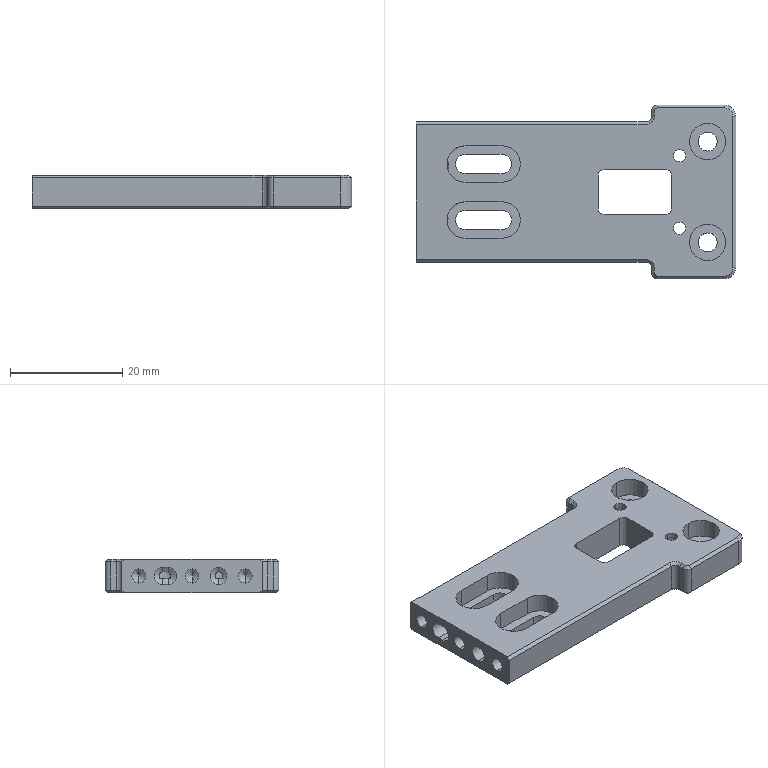Part | 1 solid | 112 faces | box 57 x 31 x 6 mm | volume 7187 mm3 | plane 46 | cylinder 44 | cone 22 | commonest cylinder face diameters 2 x8 3 x8 3.4 x8 6.5 x8 2.5 x6 2.2 x4